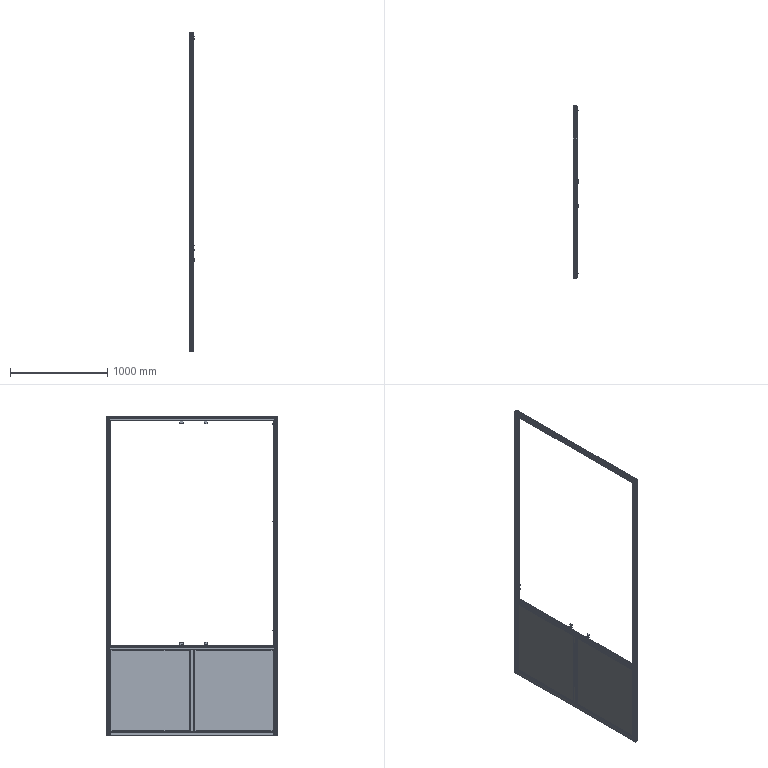Part | SolidWorks | features ReferencePattern 36, LocalLPattern 5, MirrorCompFeat 1 | 128 solids | 5358 faces | volume 15054110 mm3 | plane 3578 | cylinder 1360 | cone 380 | spline 40 | commonest cylinder face diameters 0.562 x160 8 x136 10 x96 6.8 x90 6.6 x80 2 x76